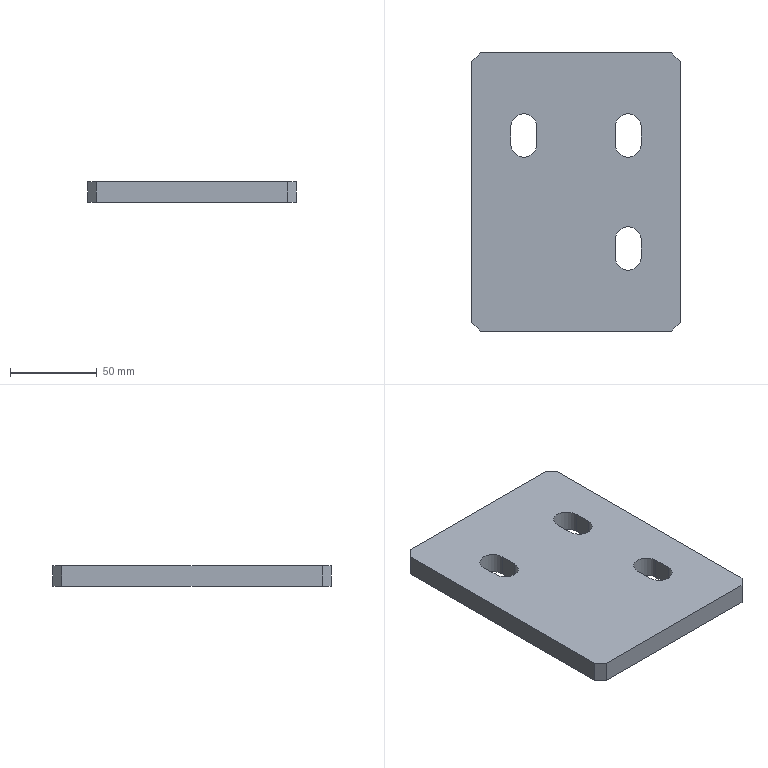Part | STEP file | Stair base plate 2-1 | 1 solid | 22 faces | box 120 x 160 x 12 mm | volume 218038 mm3 | plane 16 | cylinder 6 | commonest cylinder face diameters 15 x6